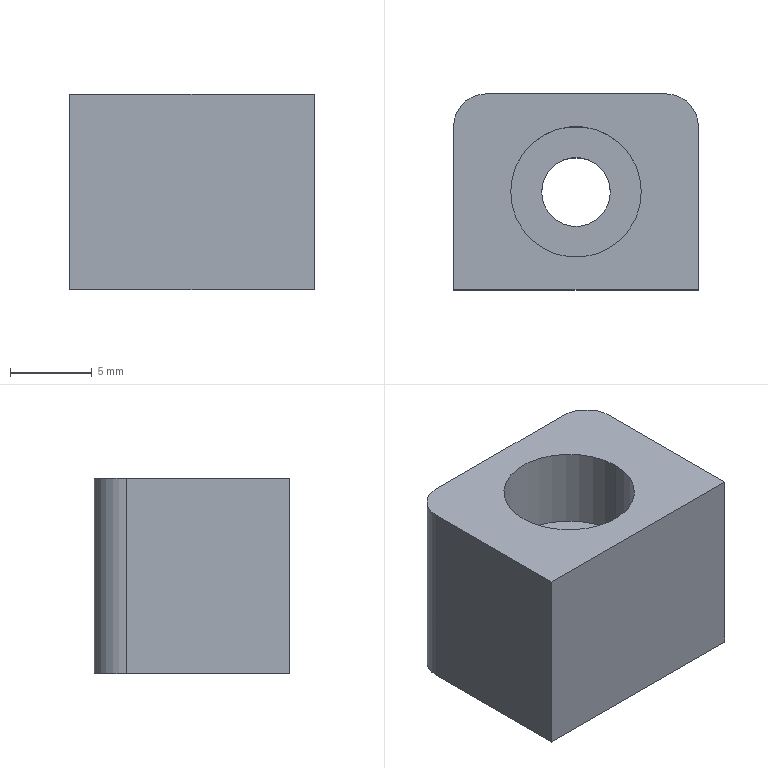Part | SolidWorks | features BaseBody 1 | 1 solid | 13 faces | box 15 x 12 x 12 mm | volume 1791 mm3 | plane 7 | cylinder 6 | commonest cylinder face diameters 4 x2 4.2 x2 8 x2
STEP:
#1=CARTESIAN_POINT('',(-676.631,766.711,328.732));
#2=VERTEX_POINT('',#1);
#3=CARTESIAN_POINT('',(-674.631,768.711,328.732));
#4=VERTEX_POINT('',#3);
#5=CARTESIAN_POINT('',(-674.631,766.711,328.732));
#6=DIRECTION('',(0.,0.,-1.));
#7=DIRECTION('',(-1.,0.,0.));
#8=AXIS2_PLACEMENT_3D('',#5,#6,#7);
#9=CIRCLE('',#8,2.);
#10=EDGE_CURVE('',#2,#4,#9,.T.);
#11=ORIENTED_EDGE('',*,*,#10,.T.);
#12=CARTESIAN_POINT('',(-674.631,768.711,316.732));
#13=VERTEX_POINT('',#12);
#14=CARTESIAN_POINT('',(-674.631,768.711,316.732));
#15=DIRECTION('',(0.,0.,1.));
#16=VECTOR('',#15,1000.);
#17=LINE('',#14,#16);
#18=EDGE_CURVE('',#13,#4,#17,.T.);
#19=ORIENTED_EDGE('',*,*,#18,.F.);
#20=CARTESIAN_POINT('',(-676.631,766.711,316.732));
#21=VERTEX_POINT('',#20);
#22=CARTESIAN_POINT('',(-674.631,766.711,316.732));
#23=DIRECTION('',(0.,0.,1.));
#24=DIRECTION('',(0.,1.,0.));
#25=AXIS2_PLACEMENT_3D('',#22,#23,#24);
#26=CIRCLE('',#25,2.);
#27=EDGE_CURVE('',#13,#21,#26,.T.);
#28=ORIENTED_EDGE('',*,*,#27,.T.);
#29=CARTESIAN_POINT('',(-676.631,766.711,328.732));
#30=DIRECTION('',(0.,0.,-1.));
#31=VECTOR('',#30,1000.);
#32=LINE('',#29,#31);
#33=EDGE_CURVE('',#2,#21,#32,.T.);
#34=ORIENTED_EDGE('',*,*,#33,.F.);
#35=EDGE_LOOP('',(#11,#19,#28,#34));
#36=FACE_OUTER_BOUND('',#35,.T.);
#37=CARTESIAN_POINT('',(-674.631,766.711,344.375));
#38=DIRECTION('',(0.,0.,-1.));
#39=DIRECTION('',(1.,0.,0.));
#40=AXIS2_PLACEMENT_3D('',#37,#38,#39);
#41=CYLINDRICAL_SURFACE('',#40,2.);
#42=ADVANCED_FACE('',(#36),#41,.T.);
#43=CARTESIAN_POINT('',(-676.631,756.711,316.732));
#44=VERTEX_POINT('',#43);
#45=CARTESIAN_POINT('',(-676.631,756.711,328.732));
#46=VERTEX_POINT('',#45);
#47=CARTESIAN_POINT('',(-676.631,756.711,316.732));
#48=DIRECTION('',(0.,0.,1.));
#49=VECTOR('',#48,1000.);
#50=LINE('',#47,#49);
#51=EDGE_CURVE('',#44,#46,#50,.T.);
#52=ORIENTED_EDGE('',*,*,#51,.T.);
#53=CARTESIAN_POINT('',(-676.631,756.711,328.732));
#54=DIRECTION('',(0.,1.,0.));
#55=VECTOR('',#54,1000.);
#56=LINE('',#53,#55);
#57=EDGE_CURVE('',#46,#2,#56,.T.);
#58=ORIENTED_EDGE('',*,*,#57,.T.);
#59=ORIENTED_EDGE('',*,*,#33,.T.);
#60=CARTESIAN_POINT('',(-676.631,766.711,316.732));
#61=DIRECTION('',(0.,-1.,0.));
#62=VECTOR('',#61,1000.);
#63=LINE('',#60,#62);
#64=EDGE_CURVE('',#21,#44,#63,.T.);
#65=ORIENTED_EDGE('',*,*,#64,.T.);
#66=EDGE_LOOP('',(#52,#58,#59,#65));
#67=FACE_OUTER_BOUND('',#66,.T.);
#68=CARTESIAN_POINT('',(-676.631,768.711,316.732));
#69=DIRECTION('',(-1.,0.,0.));
#70=DIRECTION('',(0.,1.,0.));
#71=AXIS2_PLACEMENT_3D('',#68,#69,#70);
#72=PLANE('',#71);
#73=ADVANCED_FACE('',(#67),#72,.T.);
#74=CARTESIAN_POINT('',(-661.631,756.711,316.732));
#75=VERTEX_POINT('',#74);
#76=CARTESIAN_POINT('',(-676.631,756.711,316.732));
#77=DIRECTION('',(1.,0.,0.));
#78=VECTOR('',#77,1000.);
#79=LINE('',#76,#78);
#80=EDGE_CURVE('',#44,#75,#79,.T.);
#81=ORIENTED_EDGE('',*,*,#80,.F.);
#82=ORIENTED_EDGE('',*,*,#64,.F.);
#83=ORIENTED_EDGE('',*,*,#27,.F.);
#84=CARTESIAN_POINT('',(-663.631,768.711,316.732));
#85=VERTEX_POINT('',#84);
#86=CARTESIAN_POINT('',(-663.631,768.711,316.732));
#87=DIRECTION('',(-1.,0.,0.));
#88=VECTOR('',#87,1000.);
#89=LINE('',#86,#88);
#90=EDGE_CURVE('',#85,#13,#89,.T.);
#91=ORIENTED_EDGE('',*,*,#90,.F.);
#92=CARTESIAN_POINT('',(-661.631,766.711,316.732));
#93=VERTEX_POINT('',#92);
#94=CARTESIAN_POINT('',(-663.631,766.711,316.732));
#95=DIRECTION('',(0.,0.,1.));
#96=DIRECTION('',(1.,0.,0.));
#97=AXIS2_PLACEMENT_3D('',#94,#95,#96);
#98=CIRCLE('',#97,2.);
#99=EDGE_CURVE('',#93,#85,#98,.T.);
#100=ORIENTED_EDGE('',*,*,#99,.F.);
#101=CARTESIAN_POINT('',(-661.631,756.711,316.732));
#102=DIRECTION('',(0.,1.,0.));
#103=VECTOR('',#102,1000.);
#104=LINE('',#101,#103);
#105=EDGE_CURVE('',#75,#93,#104,.T.);
#106=ORIENTED_EDGE('',*,*,#105,.F.);
#107=EDGE_LOOP('',(#81,#82,#83,#91,#100,#106));
#108=FACE_OUTER_BOUND('',#107,.T.);
#109=CARTESIAN_POINT('',(-667.031,762.711,316.732));
#110=VERTEX_POINT('',#109);
#111=CARTESIAN_POINT('',(-671.231,762.711,316.732));
#112=VERTEX_POINT('',#111);
#113=CARTESIAN_POINT('',(-669.131,762.711,316.732));
#114=DIRECTION('',(0.,0.,-1.));
#115=DIRECTION('',(1.,0.,0.));
#116=AXIS2_PLACEMENT_3D('',#113,#114,#115);
#117=CIRCLE('',#116,2.1);
#118=EDGE_CURVE('',#110,#112,#117,.T.);
#119=ORIENTED_EDGE('',*,*,#118,.F.);
#120=CARTESIAN_POINT('',(-669.131,762.711,316.732));
#121=DIRECTION('',(0.,0.,-1.));
#122=DIRECTION('',(-1.,0.,0.));
#123=AXIS2_PLACEMENT_3D('',#120,#121,#122);
#124=CIRCLE('',#123,2.1);
#125=EDGE_CURVE('',#112,#110,#124,.T.);
#126=ORIENTED_EDGE('',*,*,#125,.F.);
#127=EDGE_LOOP('',(#119,#126));
#128=FACE_BOUND('',#127,.T.);
#129=CARTESIAN_POINT('',(-637.082,1330.486,316.732));
#130=DIRECTION('',(0.,0.,1.));
#131=DIRECTION('',(-1.,0.,0.));
#132=AXIS2_PLACEMENT_3D('',#129,#130,#131);
#133=PLANE('',#132);
#134=ADVANCED_FACE('',(#108,#128),#133,.F.);
#135=CARTESIAN_POINT('',(-661.631,756.711,328.732));
#136=VERTEX_POINT('',#135);
#137=CARTESIAN_POINT('',(-661.631,756.711,316.732));
#138=DIRECTION('',(0.,0.,1.));
#139=VECTOR('',#138,1000.);
#140=LINE('',#137,#139);
#141=EDGE_CURVE('',#75,#136,#140,.T.);
#142=ORIENTED_EDGE('',*,*,#141,.F.);
#143=ORIENTED_EDGE('',*,*,#105,.T.);
#144=CARTESIAN_POINT('',(-661.631,766.711,328.732));
#145=VERTEX_POINT('',#144);
#146=CARTESIAN_POINT('',(-661.631,766.711,316.732));
#147=DIRECTION('',(0.,0.,1.));
#148=VECTOR('',#147,1000.);
#149=LINE('',#146,#148);
#150=EDGE_CURVE('',#93,#145,#149,.T.);
#151=ORIENTED_EDGE('',*,*,#150,.T.);
#152=CARTESIAN_POINT('',(-661.631,766.711,328.732));
#153=DIRECTION('',(0.,-1.,0.));
#154=VECTOR('',#153,1000.);
#155=LINE('',#152,#154);
#156=EDGE_CURVE('',#145,#136,#155,.T.);
#157=ORIENTED_EDGE('',*,*,#156,.T.);
#158=EDGE_LOOP('',(#142,#143,#151,#157));
#159=FACE_OUTER_BOUND('',#158,.T.);
#160=CARTESIAN_POINT('',(-661.631,756.711,316.732));
#161=DIRECTION('',(1.,0.,0.));
#162=DIRECTION('',(0.,-1.,0.));
#163=AXIS2_PLACEMENT_3D('',#160,#161,#162);
#164=PLANE('',#163);
#165=ADVANCED_FACE('',(#159),#164,.T.);
#166=ORIENTED_EDGE('',*,*,#10,.F.);
#167=ORIENTED_EDGE('',*,*,#57,.F.);
#168=CARTESIAN_POINT('',(-661.631,756.711,328.732));
#169=DIRECTION('',(-1.,0.,0.));
#170=VECTOR('',#169,1000.);
#171=LINE('',#168,#170);
#172=EDGE_CURVE('',#136,#46,#171,.T.);
#173=ORIENTED_EDGE('',*,*,#172,.F.);
#174=ORIENTED_EDGE('',*,*,#156,.F.);
#175=CARTESIAN_POINT('',(-663.631,768.711,328.732));
#176=VERTEX_POINT('',#175);
#177=CARTESIAN_POINT('',(-663.631,766.711,328.732));
#178=DIRECTION('',(0.,0.,-1.));
#179=DIRECTION('',(0.,1.,0.));
#180=AXIS2_PLACEMENT_3D('',#177,#178,#179);
#181=CIRCLE('',#180,2.);
#182=EDGE_CURVE('',#176,#145,#181,.T.);
#183=ORIENTED_EDGE('',*,*,#182,.F.);
#184=CARTESIAN_POINT('',(-674.631,768.711,328.732));
#185=DIRECTION('',(1.,0.,0.));
#186=VECTOR('',#185,1000.);
#187=LINE('',#184,#186);
#188=EDGE_CURVE('',#4,#176,#187,.T.);
#189=ORIENTED_EDGE('',*,*,#188,.F.);
#190=EDGE_LOOP('',(#166,#167,#173,#174,#183,#189));
#191=FACE_OUTER_BOUND('',#190,.T.);
#192=CARTESIAN_POINT('',(-665.131,762.711,328.732));
#193=VERTEX_POINT('',#192);
#194=CARTESIAN_POINT('',(-673.131,762.711,328.732));
#195=VERTEX_POINT('',#194);
#196=CARTESIAN_POINT('',(-669.131,762.711,328.732));
#197=DIRECTION('',(0.,0.,1.));
#198=DIRECTION('',(1.,0.,0.));
#199=AXIS2_PLACEMENT_3D('',#196,#197,#198);
#200=CIRCLE('',#199,4.);
#201=EDGE_CURVE('',#193,#195,#200,.T.);
#202=ORIENTED_EDGE('',*,*,#201,.F.);
#203=CARTESIAN_POINT('',(-669.131,762.711,328.732));
#204=DIRECTION('',(0.,0.,1.));
#205=DIRECTION('',(-1.,0.,0.));
#206=AXIS2_PLACEMENT_3D('',#203,#204,#205);
#207=CIRCLE('',#206,4.);
#208=EDGE_CURVE('',#195,#193,#207,.T.);
#209=ORIENTED_EDGE('',*,*,#208,.F.);
#210=EDGE_LOOP('',(#202,#209));
#211=FACE_BOUND('',#210,.T.);
#212=CARTESIAN_POINT('',(-637.082,1330.486,328.732));
#213=DIRECTION('',(0.,0.,1.));
#214=DIRECTION('',(-1.,0.,0.));
#215=AXIS2_PLACEMENT_3D('',#212,#213,#214);
#216=PLANE('',#215);
#217=ADVANCED_FACE('',(#191,#211),#216,.T.);
#218=ORIENTED_EDGE('',*,*,#18,.T.);
#219=ORIENTED_EDGE('',*,*,#188,.T.);
#220=CARTESIAN_POINT('',(-663.631,768.711,328.732));
#221=DIRECTION('',(0.,0.,-1.));
#222=VECTOR('',#221,1000.);
#223=LINE('',#220,#222);
#224=EDGE_CURVE('',#176,#85,#223,.T.);
#225=ORIENTED_EDGE('',*,*,#224,.T.);
#226=ORIENTED_EDGE('',*,*,#90,.T.);
#227=EDGE_LOOP('',(#218,#219,#225,#226));
#228=FACE_OUTER_BOUND('',#227,.T.);
#229=CARTESIAN_POINT('',(-661.631,768.711,316.732));
#230=DIRECTION('',(0.,1.,0.));
#231=DIRECTION('',(0.,0.,-1.));
#232=AXIS2_PLACEMENT_3D('',#229,#230,#231);
#233=PLANE('',#232);
#234=ADVANCED_FACE('',(#228),#233,.T.);
#235=ORIENTED_EDGE('',*,*,#182,.T.);
#236=ORIENTED_EDGE('',*,*,#150,.F.);
#237=ORIENTED_EDGE('',*,*,#99,.T.);
#238=ORIENTED_EDGE('',*,*,#224,.F.);
#239=EDGE_LOOP('',(#235,#236,#237,#238));
#240=FACE_OUTER_BOUND('',#239,.T.);
#241=CARTESIAN_POINT('',(-663.631,766.711,344.375));
#242=DIRECTION('',(0.,0.,-1.));
#243=DIRECTION('',(1.,0.,0.));
#244=AXIS2_PLACEMENT_3D('',#241,#242,#243);
#245=CYLINDRICAL_SURFACE('',#244,2.);
#246=ADVANCED_FACE('',(#240),#245,.T.);
#247=ORIENTED_EDGE('',*,*,#172,.T.);
#248=ORIENTED_EDGE('',*,*,#51,.F.);
#249=ORIENTED_EDGE('',*,*,#80,.T.);
#250=ORIENTED_EDGE('',*,*,#141,.T.);
#251=EDGE_LOOP('',(#247,#248,#249,#250));
#252=FACE_OUTER_BOUND('',#251,.T.);
#253=CARTESIAN_POINT('',(-676.631,756.711,316.732));
#254=DIRECTION('',(0.,-1.,0.));
#255=DIRECTION('',(-1.,0.,0.));
#256=AXIS2_PLACEMENT_3D('',#253,#254,#255);
#257=PLANE('',#256);
#258=ADVANCED_FACE('',(#252),#257,.T.);
#259=CARTESIAN_POINT('',(-665.131,762.711,323.732));
#260=VERTEX_POINT('',#259);
#261=CARTESIAN_POINT('',(-673.131,762.711,323.732));
#262=VERTEX_POINT('',#261);
#263=CARTESIAN_POINT('',(-669.131,762.711,323.732));
#264=DIRECTION('',(0.,0.,-1.));
#265=DIRECTION('',(1.,0.,0.));
#266=AXIS2_PLACEMENT_3D('',#263,#264,#265);
#267=CIRCLE('',#266,4.);
#268=EDGE_CURVE('',#260,#262,#267,.T.);
#269=ORIENTED_EDGE('',*,*,#268,.T.);
#270=CARTESIAN_POINT('',(-673.131,762.711,323.732));
#271=DIRECTION('',(0.,0.,1.));
#272=VECTOR('',#271,1000.);
#273=LINE('',#270,#272);
#274=EDGE_CURVE('',#262,#195,#273,.T.);
#275=ORIENTED_EDGE('',*,*,#274,.T.);
#276=ORIENTED_EDGE('',*,*,#208,.T.);
#277=CARTESIAN_POINT('',(-665.131,762.711,328.732));
#278=DIRECTION('',(0.,0.,-1.));
#279=VECTOR('',#278,1000.);
#280=LINE('',#277,#279);
#281=EDGE_CURVE('',#193,#260,#280,.T.);
#282=ORIENTED_EDGE('',*,*,#281,.T.);
#283=EDGE_LOOP('',(#269,#275,#276,#282));
#284=FACE_OUTER_BOUND('',#283,.T.);
#285=CARTESIAN_POINT('',(-669.131,762.711,328.732));
#286=DIRECTION('',(0.,0.,1.));
#287=DIRECTION('',(-1.,0.,0.));
#288=AXIS2_PLACEMENT_3D('',#285,#286,#287);
#289=CYLINDRICAL_SURFACE('',#288,4.);
#290=ADVANCED_FACE('',(#284),#289,.F.);
#291=CARTESIAN_POINT('',(-669.131,762.711,323.732));
#292=DIRECTION('',(0.,0.,-1.));
#293=DIRECTION('',(-1.,0.,0.));
#294=AXIS2_PLACEMENT_3D('',#291,#292,#293);
#295=CIRCLE('',#294,4.);
#296=EDGE_CURVE('',#262,#260,#295,.T.);
#297=ORIENTED_EDGE('',*,*,#296,.T.);
#298=ORIENTED_EDGE('',*,*,#281,.F.);
#299=ORIENTED_EDGE('',*,*,#201,.T.);
#300=ORIENTED_EDGE('',*,*,#274,.F.);
#301=EDGE_LOOP('',(#297,#298,#299,#300));
#302=FACE_OUTER_BOUND('',#301,.T.);
#303=CARTESIAN_POINT('',(-669.131,762.711,328.732));
#304=DIRECTION('',(0.,0.,1.));
#305=DIRECTION('',(-1.,0.,0.));
#306=AXIS2_PLACEMENT_3D('',#303,#304,#305);
#307=CYLINDRICAL_SURFACE('',#306,4.);
#308=ADVANCED_FACE('',(#302),#307,.F.);
#309=ORIENTED_EDGE('',*,*,#296,.F.);
#310=ORIENTED_EDGE('',*,*,#268,.F.);
#311=EDGE_LOOP('',(#309,#310));
#312=FACE_OUTER_BOUND('',#311,.T.);
#313=CARTESIAN_POINT('',(-671.231,762.711,323.732));
#314=VERTEX_POINT('',#313);
#315=CARTESIAN_POINT('',(-667.031,762.711,323.732));
#316=VERTEX_POINT('',#315);
#317=CARTESIAN_POINT('',(-669.131,762.711,323.732));
#318=DIRECTION('',(0.,0.,1.));
#319=DIRECTION('',(-1.,0.,0.));
#320=AXIS2_PLACEMENT_3D('',#317,#318,#319);
#321=CIRCLE('',#320,2.1);
#322=EDGE_CURVE('',#314,#316,#321,.T.);
#323=ORIENTED_EDGE('',*,*,#322,.F.);
#324=CARTESIAN_POINT('',(-669.131,762.711,323.732));
#325=DIRECTION('',(0.,0.,1.));
#326=DIRECTION('',(1.,0.,0.));
#327=AXIS2_PLACEMENT_3D('',#324,#325,#326);
#328=CIRCLE('',#327,2.1);
#329=EDGE_CURVE('',#316,#314,#328,.T.);
#330=ORIENTED_EDGE('',*,*,#329,.F.);
#331=EDGE_LOOP('',(#323,#330));
#332=FACE_BOUND('',#331,.T.);
#333=CARTESIAN_POINT('',(-637.082,1330.486,323.732));
#334=DIRECTION('',(0.,0.,1.));
#335=DIRECTION('',(-1.,0.,0.));
#336=AXIS2_PLACEMENT_3D('',#333,#334,#335);
#337=PLANE('',#336);
#338=ADVANCED_FACE('',(#312,#332),#337,.T.);
#339=ORIENTED_EDGE('',*,*,#125,.T.);
#340=CARTESIAN_POINT('',(-667.031,762.711,316.732));
#341=DIRECTION('',(0.,0.,1.));
#342=VECTOR('',#341,1000.);
#343=LINE('',#340,#342);
#344=EDGE_CURVE('',#110,#316,#343,.T.);
#345=ORIENTED_EDGE('',*,*,#344,.T.);
#346=ORIENTED_EDGE('',*,*,#329,.T.);
#347=CARTESIAN_POINT('',(-671.231,762.711,323.732));
#348=DIRECTION('',(0.,0.,-1.));
#349=VECTOR('',#348,1000.);
#350=LINE('',#347,#349);
#351=EDGE_CURVE('',#314,#112,#350,.T.);
#352=ORIENTED_EDGE('',*,*,#351,.T.);
#353=EDGE_LOOP('',(#339,#345,#346,#352));
#354=FACE_OUTER_BOUND('',#353,.T.);
#355=CARTESIAN_POINT('',(-669.131,762.711,316.732));
#356=DIRECTION('',(0.,0.,1.));
#357=DIRECTION('',(-1.,0.,0.));
#358=AXIS2_PLACEMENT_3D('',#355,#356,#357);
#359=CYLINDRICAL_SURFACE('',#358,2.1);
#360=ADVANCED_FACE('',(#354),#359,.F.);
#361=ORIENTED_EDGE('',*,*,#118,.T.);
#362=ORIENTED_EDGE('',*,*,#351,.F.);
#363=ORIENTED_EDGE('',*,*,#322,.T.);
#364=ORIENTED_EDGE('',*,*,#344,.F.);
#365=EDGE_LOOP('',(#361,#362,#363,#364));
#366=FACE_OUTER_BOUND('',#365,.T.);
#367=CARTESIAN_POINT('',(-669.131,762.711,316.732));
#368=DIRECTION('',(0.,0.,1.));
#369=DIRECTION('',(-1.,0.,0.));
#370=AXIS2_PLACEMENT_3D('',#367,#368,#369);
#371=CYLINDRICAL_SURFACE('',#370,2.1);
#372=ADVANCED_FACE('',(#366),#371,.F.);
#373=CLOSED_SHELL('',(#42,#73,#134,#165,#217,#234,#246,#258,#290,#308,#338,#360,#372));
#374=MANIFOLD_SOLID_BREP('',#373);
#375=CARTESIAN_POINT('',(0.,0.,0.));
#376=DIRECTION('',(0.,0.,1.));
#377=DIRECTION('',(1.,0.,0.));
#378=AXIS2_PLACEMENT_3D('',#375,#376,#377);
#379=(LENGTH_UNIT()NAMED_UNIT(*)SI_UNIT(.MILLI.,.METRE.));
#380=UNCERTAINTY_MEASURE_WITH_UNIT(LENGTH_MEASURE(0.00001),#379,'','');
#381=(NAMED_UNIT(*)PLANE_ANGLE_UNIT()SI_UNIT($,.RADIAN.));
#382=(NAMED_UNIT(*)SI_UNIT($,.STERADIAN.)SOLID_ANGLE_UNIT());
#383=(GEOMETRIC_REPRESENTATION_CONTEXT(3)GLOBAL_UNCERTAINTY_ASSIGNED_CONTEXT((#380))GLOBAL_UNIT_ASSIGNED_CONTEXT((#379,#381,#382))REPRESENTATION_CONTEXT('',''));
#384=ADVANCED_BREP_SHAPE_REPRESENTATION('',(#374,#378),#383);